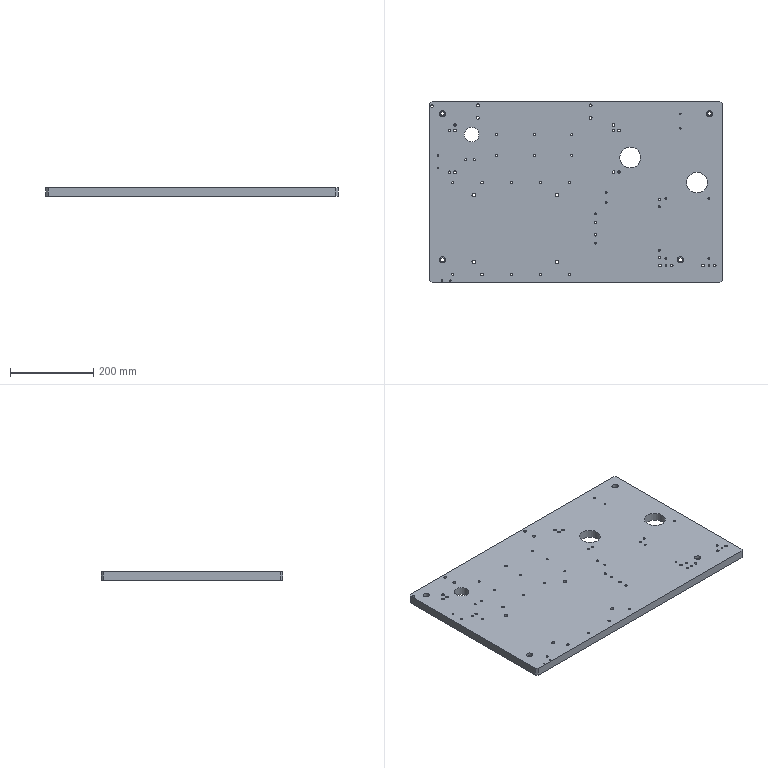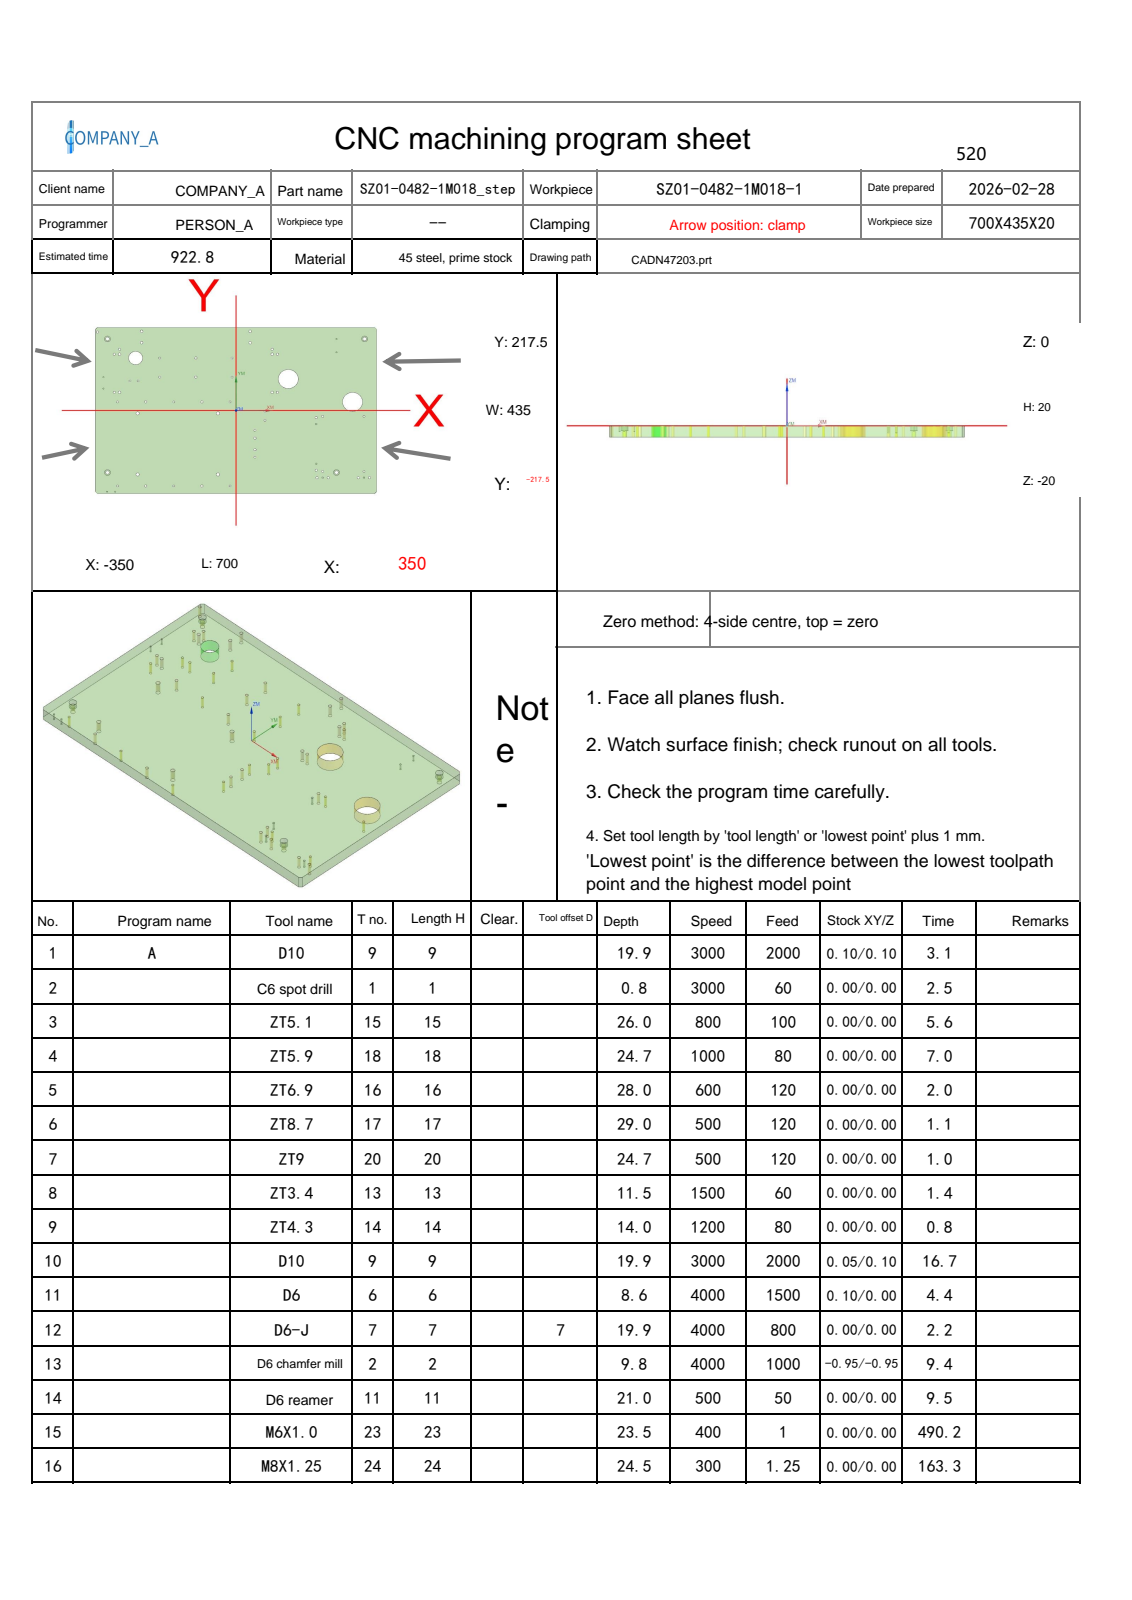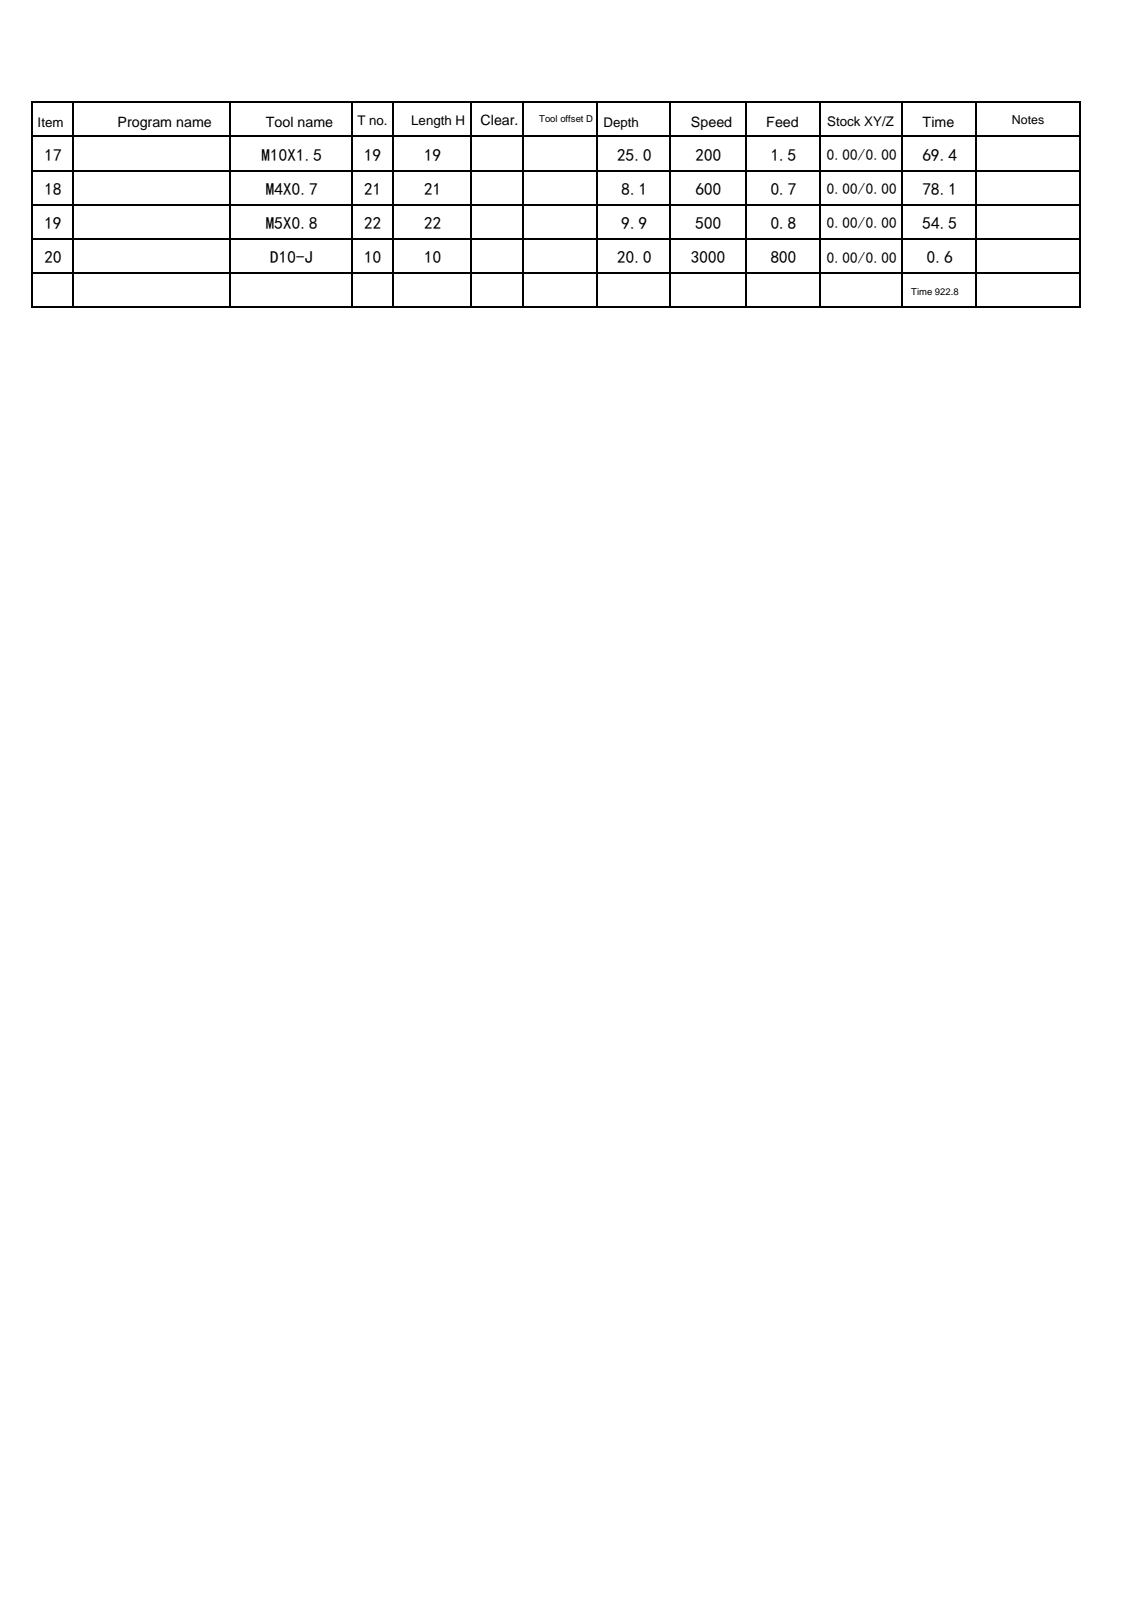NC program | NX | posted by the shop | part box 700 x 435 x 20 mm
Lines 1 to 1190 of 5271:
%
O0001
(Machine time: 1737.83 MIN)
(===Total Tool:19===)
(T9=D10     D=10.  R=0.   D-  H09 Z=-19.9 )
(T1=C6 spot drill   D=6.   R=0.   D-  H01 Z=-0.8  )
(T15=ZT5.1  D=5.1  DR_a=118 D-  H15 Z=-26.  )
(T18=ZT5.9  D=5.9  DR_a=120 D-  H18 Z=-24.7 )
(T16=ZT6.9  D=6.9  DR_a=120 D-  H16 Z=-28.  )
(T17=ZT8.7  D=8.7  DR_a=118 D-  H17 Z=-29.  )
(T20=ZT9    D=9.   DR_a=118 D-  H20 Z=-24.7 )
(T13=ZT3.4  D=3.4  DR_a=118 D-  H13 Z=-11.5 )
(T14=ZT4.3  D=4.3  DR_a=118 D-  H14 Z=-14.  )
(T6=D6      D=6.   R=0.   D-  H06 Z=-8.6  )
(T7=D6-J    D=6.   R=0.   D7  H07 Z=-19.9 )
(T2=D6 chamfer mill   D=6.   R=0.   D-  H02 Z=-9.8  )
(T11=D6 reamer   D=6.   DR_a=180 D-  H11 Z=-21.  )
(T23=M6X1.0 D=5.   DR_a=180 D-  H23 Z=-23.5 )
(T24=M8X1.25 D=6.8  DR_a=180 D-  H24 Z=-24.5 )
(T19=M10X1.5 D=8.5  DR_a=180 D-  H19 Z=-25.  )
(T21=M4X0.7 D=3.3  DR_a=180 D-  H21 Z=-8.1  )
(T22=M5X0.8 D=4.2  DR_a=180 D-  H22 Z=-9.9  )
(T10=D10-J  D=10.  R=0.   D-  H10 Z=-20.  )
G80 G90 G17 G49 G40
G91 G28 Z0
M01
N1 T09 M06
(D10  D=10. R=0. H=09 ce=0.10 di=0.10)
G00 G90 G54 X342.242 Y227.47 M03 S3000
G43 H09 Z50.
M08
Z-.35
G01 X348.606 Y221.106 F2000.
X353.606 Y216.106
X359.97 Y209.742
G00 Z-.7
G01 X353.606 Y216.106
X348.606 Y221.106
X342.242 Y227.47
G00 Z-1.05
G01 X348.606 Y221.106
X353.606 Y216.106
X359.97 Y209.742
G00 Z-1.4
G01 X353.606 Y216.106
X348.606 Y221.106
X342.242 Y227.47
G00 Z-1.75
G01 X348.606 Y221.106
X353.606 Y216.106
X359.97 Y209.742
G00 Z-2.1
G01 X353.606 Y216.106
X348.606 Y221.106
X342.242 Y227.47
G00 Z-2.45
G01 X348.606 Y221.106
X353.606 Y216.106
X359.97 Y209.742
G00 Z-2.8
G01 X353.606 Y216.106
X348.606 Y221.106
X342.242 Y227.47
G00 Z-3.15
G01 X348.606 Y221.106
X353.606 Y216.106
X359.97 Y209.742
G00 Z-3.5
G01 X353.606 Y216.106
X348.606 Y221.106
X342.242 Y227.47
G00 Z-3.85
G01 X348.606 Y221.106
X353.606 Y216.106
X359.97 Y209.742
G00 Z-4.2
G01 X353.606 Y216.106
X348.606 Y221.106
X342.242 Y227.47
G00 Z-4.55
G01 X348.606 Y221.106
X353.606 Y216.106
X359.97 Y209.742
G00 Z-4.9
G01 X353.606 Y216.106
X348.606 Y221.106
X342.242 Y227.47
G00 Z-5.25
G01 X348.606 Y221.106
X353.606 Y216.106
X359.97 Y209.742
G00 Z-5.6
G01 X353.606 Y216.106
X348.606 Y221.106
X342.242 Y227.47
G00 Z-5.95
G01 X348.606 Y221.106
X353.606 Y216.106
X359.97 Y209.742
G00 Z-6.3
G01 X353.606 Y216.106
X348.606 Y221.106
X342.242 Y227.47
G00 Z-6.65
G01 X348.606 Y221.106
X353.606 Y216.106
X359.97 Y209.742
G00 Z-7.
G01 X353.606 Y216.106
X348.606 Y221.106
X342.242 Y227.47
G00 Z-7.35
G01 X348.606 Y221.106
X353.606 Y216.106
X359.97 Y209.742
G00 Z-7.7
G01 X353.606 Y216.106
X348.606 Y221.106
X342.242 Y227.47
G00 Z-8.05
G01 X348.606 Y221.106
X353.606 Y216.106
X359.97 Y209.742
G00 Z-8.4
G01 X353.606 Y216.106
X348.606 Y221.106
X342.242 Y227.47
G00 Z-8.75
G01 X348.606 Y221.106
X353.606 Y216.106
X359.97 Y209.742
G00 Z-9.1
G01 X353.606 Y216.106
X348.606 Y221.106
X342.242 Y227.47
G00 Z-9.45
G01 X348.606 Y221.106
X353.606 Y216.106
X359.97 Y209.742
G00 Z-9.8
G01 X353.606 Y216.106
X348.606 Y221.106
X342.242 Y227.47
G00 Z-10.15
G01 X348.606 Y221.106
X353.606 Y216.106
X359.97 Y209.742
G00 Z-10.5
G01 X353.606 Y216.106
X348.606 Y221.106
X342.242 Y227.47
G00 Z-10.85
G01 X348.606 Y221.106
X353.606 Y216.106
X359.97 Y209.742
G00 Z-11.2
G01 X353.606 Y216.106
X348.606 Y221.106
X342.242 Y227.47
G00 Z-11.55
G01 X348.606 Y221.106
X353.606 Y216.106
X359.97 Y209.742
G00 Z-11.9
G01 X353.606 Y216.106
X348.606 Y221.106
X342.242 Y227.47
G00 Z-12.25
G01 X348.606 Y221.106
X353.606 Y216.106
X359.97 Y209.742
G00 Z-12.6
G01 X353.606 Y216.106
X348.606 Y221.106
X342.242 Y227.47
G00 Z-12.95
G01 X348.606 Y221.106
X353.606 Y216.106
X359.97 Y209.742
G00 Z-13.3
G01 X353.606 Y216.106
X348.606 Y221.106
X342.242 Y227.47
G00 Z-13.65
G01 X348.606 Y221.106
X353.606 Y216.106
X359.97 Y209.742
G00 Z-14.
G01 X353.606 Y216.106
X348.606 Y221.106
X342.242 Y227.47
G00 Z-14.35
G01 X348.606 Y221.106
X353.606 Y216.106
X359.97 Y209.742
G00 Z-14.7
G01 X353.606 Y216.106
X348.606 Y221.106
X342.242 Y227.47
G00 Z-15.05
G01 X348.606 Y221.106
X353.606 Y216.106
X359.97 Y209.742
G00 Z-15.4
G01 X353.606 Y216.106
X348.606 Y221.106
X342.242 Y227.47
G00 Z-15.75
G01 X348.606 Y221.106
X353.606 Y216.106
X359.97 Y209.742
G00 Z-16.1
G01 X353.606 Y216.106
X348.606 Y221.106
X342.242 Y227.47
G00 Z-16.45
G01 X348.606 Y221.106
X353.606 Y216.106
X359.97 Y209.742
G00 Z-16.8
G01 X353.606 Y216.106
X348.606 Y221.106
X342.242 Y227.47
G00 Z-17.15
G01 X348.606 Y221.106
X353.606 Y216.106
X359.97 Y209.742
G00 Z-17.5
G01 X353.606 Y216.106
X348.606 Y221.106
X342.242 Y227.47
G00 Z-17.85
G01 X348.606 Y221.106
X353.606 Y216.106
X359.97 Y209.742
G00 Z-18.2
G01 X353.606 Y216.106
X348.606 Y221.106
X342.242 Y227.47
G00 Z-18.55
G01 X348.606 Y221.106
X353.606 Y216.106
X359.97 Y209.742
G00 Z-18.9
G01 X353.606 Y216.106
X348.606 Y221.106
X342.242 Y227.47
G00 Z-19.25
G01 X348.606 Y221.106
X353.606 Y216.106
X359.97 Y209.742
G00 Z-19.6
G01 X353.606 Y216.106
X348.606 Y221.106
X342.242 Y227.47
G00 Z-19.9
G01 X348.606 Y221.106
X353.606 Y216.106
X359.97 Y209.742
G00 Z50.
Y-209.742
Z-.35
G01 X353.606 Y-216.106
X348.606 Y-221.106
X342.242 Y-227.47
G00 Z-.7
G01 X348.606 Y-221.106
X353.606 Y-216.106
X359.97 Y-209.742
G00 Z-1.05
G01 X353.606 Y-216.106
X348.606 Y-221.106
X342.242 Y-227.47
G00 Z-1.4
G01 X348.606 Y-221.106
X353.606 Y-216.106
X359.97 Y-209.742
G00 Z-1.75
G01 X353.606 Y-216.106
X348.606 Y-221.106
X342.242 Y-227.47
G00 Z-2.1
G01 X348.606 Y-221.106
X353.606 Y-216.106
X359.97 Y-209.742
G00 Z-2.45
G01 X353.606 Y-216.106
X348.606 Y-221.106
X342.242 Y-227.47
G00 Z-2.8
G01 X348.606 Y-221.106
X353.606 Y-216.106
X359.97 Y-209.742
G00 Z-3.15
G01 X353.606 Y-216.106
X348.606 Y-221.106
X342.242 Y-227.47
G00 Z-3.5
G01 X348.606 Y-221.106
X353.606 Y-216.106
X359.97 Y-209.742
G00 Z-3.85
G01 X353.606 Y-216.106
X348.606 Y-221.106
X342.242 Y-227.47
G00 Z-4.2
G01 X348.606 Y-221.106
X353.606 Y-216.106
X359.97 Y-209.742
G00 Z-4.55
G01 X353.606 Y-216.106
X348.606 Y-221.106
X342.242 Y-227.47
G00 Z-4.9
G01 X348.606 Y-221.106
X353.606 Y-216.106
X359.97 Y-209.742
G00 Z-5.25
G01 X353.606 Y-216.106
X348.606 Y-221.106
X342.242 Y-227.47
G00 Z-5.6
G01 X348.606 Y-221.106
X353.606 Y-216.106
X359.97 Y-209.742
G00 Z-5.95
G01 X353.606 Y-216.106
X348.606 Y-221.106
X342.242 Y-227.47
G00 Z-6.3
G01 X348.606 Y-221.106
X353.606 Y-216.106
X359.97 Y-209.742
G00 Z-6.65
G01 X353.606 Y-216.106
X348.606 Y-221.106
X342.242 Y-227.47
G00 Z-7.
G01 X348.606 Y-221.106
X353.606 Y-216.106
X359.97 Y-209.742
G00 Z-7.35
G01 X353.606 Y-216.106
X348.606 Y-221.106
X342.242 Y-227.47
G00 Z-7.7
G01 X348.606 Y-221.106
X353.606 Y-216.106
X359.97 Y-209.742
G00 Z-8.05
G01 X353.606 Y-216.106
X348.606 Y-221.106
X342.242 Y-227.47
G00 Z-8.4
G01 X348.606 Y-221.106
X353.606 Y-216.106
X359.97 Y-209.742
G00 Z-8.75
G01 X353.606 Y-216.106
X348.606 Y-221.106
X342.242 Y-227.47
G00 Z-9.1
G01 X348.606 Y-221.106
X353.606 Y-216.106
X359.97 Y-209.742
G00 Z-9.45
G01 X353.606 Y-216.106
X348.606 Y-221.106
X342.242 Y-227.47
G00 Z-9.8
G01 X348.606 Y-221.106
X353.606 Y-216.106
X359.97 Y-209.742
G00 Z-10.15
G01 X353.606 Y-216.106
X348.606 Y-221.106
X342.242 Y-227.47
G00 Z-10.5
G01 X348.606 Y-221.106
X353.606 Y-216.106
X359.97 Y-209.742
G00 Z-10.85
G01 X353.606 Y-216.106
X348.606 Y-221.106
X342.242 Y-227.47
G00 Z-11.2
G01 X348.606 Y-221.106
X353.606 Y-216.106
X359.97 Y-209.742
G00 Z-11.55
G01 X353.606 Y-216.106
X348.606 Y-221.106
X342.242 Y-227.47
G00 Z-11.9
G01 X348.606 Y-221.106
X353.606 Y-216.106
X359.97 Y-209.742
G00 Z-12.25
G01 X353.606 Y-216.106
X348.606 Y-221.106
X342.242 Y-227.47
G00 Z-12.6
G01 X348.606 Y-221.106
X353.606 Y-216.106
X359.97 Y-209.742
G00 Z-12.95
G01 X353.606 Y-216.106
X348.606 Y-221.106
X342.242 Y-227.47
G00 Z-13.3
G01 X348.606 Y-221.106
X353.606 Y-216.106
X359.97 Y-209.742
G00 Z-13.65
G01 X353.606 Y-216.106
X348.606 Y-221.106
X342.242 Y-227.47
G00 Z-14.
G01 X348.606 Y-221.106
X353.606 Y-216.106
X359.97 Y-209.742
G00 Z-14.35
G01 X353.606 Y-216.106
X348.606 Y-221.106
X342.242 Y-227.47
G00 Z-14.7
G01 X348.606 Y-221.106
X353.606 Y-216.106
X359.97 Y-209.742
G00 Z-15.05
G01 X353.606 Y-216.106
X348.606 Y-221.106
X342.242 Y-227.47
G00 Z-15.4
G01 X348.606 Y-221.106
X353.606 Y-216.106
X359.97 Y-209.742
G00 Z-15.75
G01 X353.606 Y-216.106
X348.606 Y-221.106
X342.242 Y-227.47
G00 Z-16.1
G01 X348.606 Y-221.106
X353.606 Y-216.106
X359.97 Y-209.742
G00 Z-16.45
G01 X353.606 Y-216.106
X348.606 Y-221.106
X342.242 Y-227.47
G00 Z-16.8
G01 X348.606 Y-221.106
X353.606 Y-216.106
X359.97 Y-209.742
G00 Z-17.15
G01 X353.606 Y-216.106
X348.606 Y-221.106
X342.242 Y-227.47
G00 Z-17.5
G01 X348.606 Y-221.106
X353.606 Y-216.106
X359.97 Y-209.742
G00 Z-17.85
G01 X353.606 Y-216.106
X348.606 Y-221.106
X342.242 Y-227.47
G00 Z-18.2
G01 X348.606 Y-221.106
X353.606 Y-216.106
X359.97 Y-209.742
G00 Z-18.55
G01 X353.606 Y-216.106
X348.606 Y-221.106
X342.242 Y-227.47
G00 Z-18.9
G01 X348.606 Y-221.106
X353.606 Y-216.106
X359.97 Y-209.742
G00 Z-19.25
G01 X353.606 Y-216.106
X348.606 Y-221.106
X342.242 Y-227.47
G00 Z-19.6
G01 X348.606 Y-221.106
X353.606 Y-216.106
X359.97 Y-209.742
G00 Z-19.9
G01 X353.606 Y-216.106
X348.606 Y-221.106
X342.242 Y-227.47
G00 Z50.
X-342.242
Z-.35
G01 X-348.606 Y-221.106
X-353.606 Y-216.106
X-359.97 Y-209.742
G00 Z-.7
G01 X-353.606 Y-216.106
X-348.606 Y-221.106
X-342.242 Y-227.47
G00 Z-1.05
G01 X-348.606 Y-221.106
X-353.606 Y-216.106
X-359.97 Y-209.742
G00 Z-1.4
G01 X-353.606 Y-216.106
X-348.606 Y-221.106
X-342.242 Y-227.47
G00 Z-1.75
G01 X-348.606 Y-221.106
X-353.606 Y-216.106
X-359.97 Y-209.742
G00 Z-2.1
G01 X-353.606 Y-216.106
X-348.606 Y-221.106
X-342.242 Y-227.47
G00 Z-2.45
G01 X-348.606 Y-221.106
X-353.606 Y-216.106
X-359.97 Y-209.742
G00 Z-2.8
G01 X-353.606 Y-216.106
X-348.606 Y-221.106
X-342.242 Y-227.47
G00 Z-3.15
G01 X-348.606 Y-221.106
X-353.606 Y-216.106
X-359.97 Y-209.742
G00 Z-3.5
G01 X-353.606 Y-216.106
X-348.606 Y-221.106
X-342.242 Y-227.47
G00 Z-3.85
G01 X-348.606 Y-221.106
X-353.606 Y-216.106
X-359.97 Y-209.742
G00 Z-4.2
G01 X-353.606 Y-216.106
X-348.606 Y-221.106
X-342.242 Y-227.47
G00 Z-4.55
G01 X-348.606 Y-221.106
X-353.606 Y-216.106
X-359.97 Y-209.742
G00 Z-4.9
G01 X-353.606 Y-216.106
X-348.606 Y-221.106
X-342.242 Y-227.47
G00 Z-5.25
G01 X-348.606 Y-221.106
X-353.606 Y-216.106
X-359.97 Y-209.742
G00 Z-5.6
G01 X-353.606 Y-216.106
X-348.606 Y-221.106
X-342.242 Y-227.47
G00 Z-5.95
G01 X-348.606 Y-221.106
X-353.606 Y-216.106
X-359.97 Y-209.742
G00 Z-6.3
G01 X-353.606 Y-216.106
X-348.606 Y-221.106
X-342.242 Y-227.47
G00 Z-6.65
G01 X-348.606 Y-221.106
X-353.606 Y-216.106
X-359.97 Y-209.742
G00 Z-7.
G01 X-353.606 Y-216.106
X-348.606 Y-221.106
X-342.242 Y-227.47
G00 Z-7.35
G01 X-348.606 Y-221.106
X-353.606 Y-216.106
X-359.97 Y-209.742
G00 Z-7.7
G01 X-353.606 Y-216.106
X-348.606 Y-221.106
X-342.242 Y-227.47
G00 Z-8.05
G01 X-348.606 Y-221.106
X-353.606 Y-216.106
X-359.97 Y-209.742
G00 Z-8.4
G01 X-353.606 Y-216.106
X-348.606 Y-221.106
X-342.242 Y-227.47
G00 Z-8.75
G01 X-348.606 Y-221.106
X-353.606 Y-216.106
X-359.97 Y-209.742
G00 Z-9.1
G01 X-353.606 Y-216.106
X-348.606 Y-221.106
X-342.242 Y-227.47
G00 Z-9.45
G01 X-348.606 Y-221.106
X-353.606 Y-216.106
X-359.97 Y-209.742
G00 Z-9.8
G01 X-353.606 Y-216.106
X-348.606 Y-221.106
X-342.242 Y-227.47
G00 Z-10.15
G01 X-348.606 Y-221.106
X-353.606 Y-216.106
X-359.97 Y-209.742
G00 Z-10.5
G01 X-353.606 Y-216.106
X-348.606 Y-221.106
X-342.242 Y-227.47
G00 Z-10.85
G01 X-348.606 Y-221.106
X-353.606 Y-216.106
X-359.97 Y-209.742
G00 Z-11.2
G01 X-353.606 Y-216.106
X-348.606 Y-221.106
X-342.242 Y-227.47
G00 Z-11.55
G01 X-348.606 Y-221.106
X-353.606 Y-216.106
X-359.97 Y-209.742
G00 Z-11.9
G01 X-353.606 Y-216.106
X-348.606 Y-221.106
X-342.242 Y-227.47
G00 Z-12.25
G01 X-348.606 Y-221.106
X-353.606 Y-216.106
X-359.97 Y-209.742
G00 Z-12.6
G01 X-353.606 Y-216.106
X-348.606 Y-221.106
X-342.242 Y-227.47
G00 Z-12.95
G01 X-348.606 Y-221.106
X-353.606 Y-216.106
X-359.97 Y-209.742
G00 Z-13.3
G01 X-353.606 Y-216.106
X-348.606 Y-221.106
X-342.242 Y-227.47
G00 Z-13.65
G01 X-348.606 Y-221.106
X-353.606 Y-216.106
X-359.97 Y-209.742
G00 Z-14.
G01 X-353.606 Y-216.106
X-348.606 Y-221.106
X-342.242 Y-227.47
G00 Z-14.35
G01 X-348.606 Y-221.106
X-353.606 Y-216.106
X-359.97 Y-209.742
G00 Z-14.7
G01 X-353.606 Y-216.106
X-348.606 Y-221.106
X-342.242 Y-227.47
G00 Z-15.05
G01 X-348.606 Y-221.106
X-353.606 Y-216.106
X-359.97 Y-209.742
G00 Z-15.4
G01 X-353.606 Y-216.106
X-348.606 Y-221.106
X-342.242 Y-227.47
G00 Z-15.75
G01 X-348.606 Y-221.106
X-353.606 Y-216.106
X-359.97 Y-209.742
G00 Z-16.1
G01 X-353.606 Y-216.106
X-348.606 Y-221.106
X-342.242 Y-227.47
G00 Z-16.45
G01 X-348.606 Y-221.106
X-353.606 Y-216.106
X-359.97 Y-209.742
G00 Z-16.8
G01 X-353.606 Y-216.106
X-348.606 Y-221.106
X-342.242 Y-227.47
G00 Z-17.15
G01 X-348.606 Y-221.106
X-353.606 Y-216.106
X-359.97 Y-209.742
G00 Z-17.5
G01 X-353.606 Y-216.106
X-348.606 Y-221.106
X-342.242 Y-227.47
G00 Z-17.85
G01 X-348.606 Y-221.106
X-353.606 Y-216.106
X-359.97 Y-209.742
G00 Z-18.2
G01 X-353.606 Y-216.106
X-348.606 Y-221.106
X-342.242 Y-227.47
G00 Z-18.55
G01 X-348.606 Y-221.106
X-353.606 Y-216.106
X-359.97 Y-209.742
G00 Z-18.9
G01 X-353.606 Y-216.106
X-348.606 Y-221.106
X-342.242 Y-227.47
G00 Z-19.25
G01 X-348.606 Y-221.106
X-353.606 Y-216.106
X-359.97 Y-209.742
G00 Z-19.6
G01 X-353.606 Y-216.106
X-348.606 Y-221.106
X-342.242 Y-227.47
G00 Z-19.9
G01 X-348.606 Y-221.106
X-353.606 Y-216.106
X-359.97 Y-209.742
G00 Z50.
Y209.742
Z-.35
G01 X-353.606 Y216.106
X-348.606 Y221.106
X-342.242 Y227.47
G00 Z-.7
G01 X-348.606 Y221.106
X-353.606 Y216.106
X-359.97 Y209.742
G00 Z-1.05
G01 X-353.606 Y216.106
X-348.606 Y221.106
X-342.242 Y227.47
G00 Z-1.4
G01 X-348.606 Y221.106
X-353.606 Y216.106
X-359.97 Y209.742
G00 Z-1.75
G01 X-353.606 Y216.106
X-348.606 Y221.106
X-342.242 Y227.47
G00 Z-2.1
G01 X-348.606 Y221.106
X-353.606 Y216.106
X-359.97 Y209.742
G00 Z-2.45
G01 X-353.606 Y216.106
X-348.606 Y221.106
X-342.242 Y227.47
G00 Z-2.8
G01 X-348.606 Y221.106
X-353.606 Y216.106
X-359.97 Y209.742
G00 Z-3.15
G01 X-353.606 Y216.106
X-348.606 Y221.106
X-342.242 Y227.47
G00 Z-3.5
G01 X-348.606 Y221.106
X-353.606 Y216.106
X-359.97 Y209.742
G00 Z-3.85
G01 X-353.606 Y216.106
X-348.606 Y221.106
X-342.242 Y227.47
G00 Z-4.2
G01 X-348.606 Y221.106
X-353.606 Y216.106
X-359.97 Y209.742
G00 Z-4.55
G01 X-353.606 Y216.106
X-348.606 Y221.106
X-342.242 Y227.47
G00 Z-4.9
G01 X-348.606 Y221.106
X-353.606 Y216.106
X-359.97 Y209.742
G00 Z-5.25
G01 X-353.606 Y216.106
X-348.606 Y221.106
X-342.242 Y227.47
G00 Z-5.6
G01 X-348.606 Y221.106
X-353.606 Y216.106
X-359.97 Y209.742
G00 Z-5.95
G01 X-353.606 Y216.106
X-348.606 Y221.106
X-342.242 Y227.47
G00 Z-6.3
G01 X-348.606 Y221.106
X-353.606 Y216.106
X-359.97 Y209.742
G00 Z-6.65
G01 X-353.606 Y216.106
X-348.606 Y221.106
X-342.242 Y227.47
G00 Z-7.
G01 X-348.606 Y221.106
X-353.606 Y216.106
X-359.97 Y209.742
G00 Z-7.35
G01 X-353.606 Y216.106
X-348.606 Y221.106
X-342.242 Y227.47
G00 Z-7.7
G01 X-348.606 Y221.106
X-353.606 Y216.106
X-359.97 Y209.742
G00 Z-8.05
G01 X-353.606 Y216.106
X-348.606 Y221.106
X-342.242 Y227.47
G00 Z-8.4
G01 X-348.606 Y221.106
X-353.606 Y216.106
X-359.97 Y209.742
G00 Z-8.75
G01 X-353.606 Y216.106
X-348.606 Y221.106
X-342.242 Y227.47
G00 Z-9.1
G01 X-348.606 Y221.106
X-353.606 Y216.106
X-359.97 Y209.742
G00 Z-9.45
G01 X-353.606 Y216.106
X-348.606 Y221.106
X-342.242 Y227.47
G00 Z-9.8
G01 X-348.606 Y221.106
X-353.606 Y216.106
X-359.97 Y209.742
G00 Z-10.15
G01 X-353.606 Y216.106
X-348.606 Y221.106
X-342.242 Y227.47
G00 Z-10.5
G01 X-348.606 Y221.106
X-353.606 Y216.106
X-359.97 Y209.742
G00 Z-10.85
G01 X-353.606 Y216.106
X-348.606 Y221.106
X-342.242 Y227.47
G00 Z-11.2
G01 X-348.606 Y221.106
X-353.606 Y216.106
X-359.97 Y209.742
G00 Z-11.55
G01 X-353.606 Y216.106
X-348.606 Y221.106
X-342.242 Y227.47
G00 Z-11.9
G01 X-348.606 Y221.106
X-353.606 Y216.106
X-359.97 Y209.742
G00 Z-12.25
G01 X-353.606 Y216.106
X-348.606 Y221.106
X-342.242 Y227.47
G00 Z-12.6
G01 X-348.606 Y221.106
X-353.606 Y216.106
X-359.97 Y209.742
G00 Z-12.95
G01 X-353.606 Y216.106
X-348.606 Y221.106
X-342.242 Y227.47
G00 Z-13.3
G01 X-348.606 Y221.106
X-353.606 Y216.106
X-359.97 Y209.742
G00 Z-13.65
G01 X-353.606 Y216.106
X-348.606 Y221.106
X-342.242 Y227.47
G00 Z-14.
G01 X-348.606 Y221.106
X-353.606 Y216.106
X-359.97 Y209.742
G00 Z-14.35
G01 X-353.606 Y216.106
X-348.606 Y221.106
X-342.242 Y227.47
G00 Z-14.7
G01 X-348.606 Y221.106
X-353.606 Y216.106
X-359.97 Y209.742
G00 Z-15.05
G01 X-353.606 Y216.106
X-348.606 Y221.106
X-342.242 Y227.47
G00 Z-15.4
G01 X-348.606 Y221.106
X-353.606 Y216.106
X-359.97 Y209.742
G00 Z-15.75
G01 X-353.606 Y216.106
X-348.606 Y221.106
X-342.242 Y227.47
G00 Z-16.1
G01 X-348.606 Y221.106
X-353.606 Y216.106
X-359.97 Y209.742
G00 Z-16.45
G01 X-353.606 Y216.106
X-348.606 Y221.106
X-342.242 Y227.47
G00 Z-16.8
G01 X-348.606 Y221.106
X-353.606 Y216.106
X-359.97 Y209.742
G00 Z-17.15
G01 X-353.606 Y216.106
X-348.606 Y221.106
X-342.242 Y227.47
G00 Z-17.5
G01 X-348.606 Y221.106
X-353.606 Y216.106
X-359.97 Y209.742
G00 Z-17.85
G01 X-353.606 Y216.106
X-348.606 Y221.106
X-342.242 Y227.47
G00 Z-18.2
G01 X-348.606 Y221.106
X-353.606 Y216.106
X-359.97 Y209.742
G00 Z-18.55
G01 X-353.606 Y216.106
X-348.606 Y221.106
X-342.242 Y227.47
G00 Z-18.9
G01 X-348.606 Y221.106
X-353.606 Y216.106
X-359.97 Y209.742
G00 Z-19.25
G01 X-353.606 Y216.106
X-348.606 Y221.106
X-342.242 Y227.47
G00 Z-19.6
G01 X-348.606 Y221.106
X-353.606 Y216.106
X-359.97 Y209.742
G00 Z-19.9
G01 X-353.606 Y216.106
X-348.606 Y221.106
X-342.242 Y227.47
G00 Z50.
G91 G28 Z0.0
M05
M09
G91 G28 Z0.0
M01
N2 T01 M06
(C6 spot drill  D=6. R=0. H=01 ce=0.00 di=0.10)
G00 G90 G54 X-345. Y205.5 M03 S3000
G43 H01 Z50.
M08
G98 G81 X-345. Y205.5 Z-.8 R1. F60.
X-320. Y187.5
X-290. Y160.5
X-303. Y147.5
X-290.
X-250. Y137.5
X-235. Y177.5
Y207.5
X-190. Y137.5
X-100.
Y87.5
X-10.
Y137.5
X35. Y177.5
Y207.5
X90. Y160.5
Y147.5
X103.
X130. Y82.5
X103. Y47.5
X90.
X72. Y-1.5
Y-25.5
X47. Y-72.5
Y-52.5
X-15. Y22.5
X-45. Y-7.5
X-85. Y22.5
X-155.
X-190. Y87.5
X-244. Y77.5
X-264.
X-330. Y87.5
Y57.5
X-303. Y47.5
X-290.
X-295. Y22.5
X-225.
X-245. Y-7.5
X-320. Y-162.5
X-321. Y-212.5
X-301.
X-295. Y-197.5
X-245. Y-167.5
X-225. Y-197.5
X-155.
X-85.
X-45. Y-167.5
X-15. Y-197.5
X47. Y-122.5
Y-102.5
X199.5 Y-139.5
Y-156.5
X215.5 Y-159.5
X201.5 Y-176.
X215.5
X229.5
X250. Y-162.5
X304.5 Y-176.
X318.5
X332.5
X318.5 Y-159.5
X199.5 Y-35.5
Y-18.5
X215.5 Y-15.5
X318.5
X290. Y22.5
X250. Y152.5
Y187.5
X320.
G80
G00 Z50.
G91 G28 Z0.0
M05
M09
G91 G28 Z0.0
M01
N3 T15 M06
(ZT5.1 D=5.1 DR_a=118 H=15)
G00 G90 G54 X-295. Y-197.5 M03 S800
G43 H15 Z50.
M08
G98 G83 X-295. Y-197.5 Z-26. R1. F100. Q2.
X-155.
X-15.
X47. Y-122.5
X215.5 Y-159.5
X318.5
Y-15.5
X215.5
X72. Y-1.5
Y-25.5
X47. Y-52.5
X-15. Y22.5
X-10. Y87.5
Y137.5
X-155. Y22.5
X-190. Y87.5
Y137.5
X-244. Y77.5
X-264.
X-295. Y22.5
G80
G00 Z50.
G91 G28 Z0.0
M05
M09
G91 G28 Z0.0
M01
N4 T18 M06
(ZT5.9 D=5.9 DR_a=120 H=18)
G00 G90 G54 X332.5 Y-176. M03 S1000
G43 H18 Z50.
M08
G98 G83 X332.5 Y-176. Z-24.703 R1. F80. Q1.
X304.5
X229.5
X201.5
X199.5 Y-156.5
Y-18.5
X103. Y47.5
Y147.5
X90. Y160.5
X-100. Y137.5
Y87.5
X-85. Y22.5
X47. Y-72.5
Y-102.5
X-85. Y-197.5
X-225.
Y22.5
X-303. Y47.5
Y147.5
X-290. Y160.5
X-345. Y205.5
G80
G00 Z50.
G91 G28 Z0.0
M05
M09
G91 G28 Z0.0
M01
N5 T16 M06
(ZT6.9 D=6.9 DR_a=120 H=16)
G00 G90 G54 X-290. Y47.5 M03 S600
G43 H16 Z50.
M08
G98 G83 X-290. Y47.5 Z-28. R1. F120. Q2.
Y147.5
X-235. Y177.5
Y207.5
X35.
Y177.5
X90. Y147.5
Y47.5
G80
G00 Z50.
G91 G28 Z0.0
M05
M09
G91 G28 Z0.0
M01
N6 T17 M06
(ZT8.7 D=8.7 DR_a=118 H=17)
G00 G90 G54 X-245. Y-7.5 M03 S500
G43 H17 Z50.
M08
G98 G83 X-245. Y-7.5 Z-29. R1. F120. Q2.
Y-167.5
X-45.
Y-7.5
G80
G00 Z50.
G91 G28 Z0.0
M05
M09
G91 G28 Z0.0
M01
N7 T20 M06
(ZT9 D=9. DR_a=118 H=20)
G00 G90 G54 X320. Y187.5 M03 S500
G43 H20 Z50.
M08
G98 G83 X320. Y187.5 Z-24.704 R1. F120. Q2.
X250. Y-162.5
X-320.
Y187.5
G80
G00 Z50.
G91 G28 Z0.0
M05
M09
G91 G28 Z0.0
M01
N8 T13 M06
(ZT3.4 D=3.4 DR_a=118 H=13)
G00 G90 G54 X250. Y187.5 M03 S1500
G43 H13 Z50.
M08
G98 G83 X250. Y187.5 Z-11.5 R1. F60. Q1.
Y152.5
X-330. Y87.5
Y57.5
X-321. Y-212.5
X-301.
G80
G00 Z50.
G91 G28 Z0.0
M05
M09
G91 G28 Z0.0
M01
N9 T14 M06
(ZT4.3 D=4.3 DR_a=118 H=14)
G00 G90 G54 X199.5 Y-35.5 M03 S1200
G43 H14 Z50.
M08
G98 G83 X199.5 Y-35.5 Z-14. R1. F80. Q1.
Y-139.5
X215.5 Y-176.
X318.5
G80
G00 Z50.
G91 G28 Z0.0
M05
M09
G91 G28 Z0.0
M01